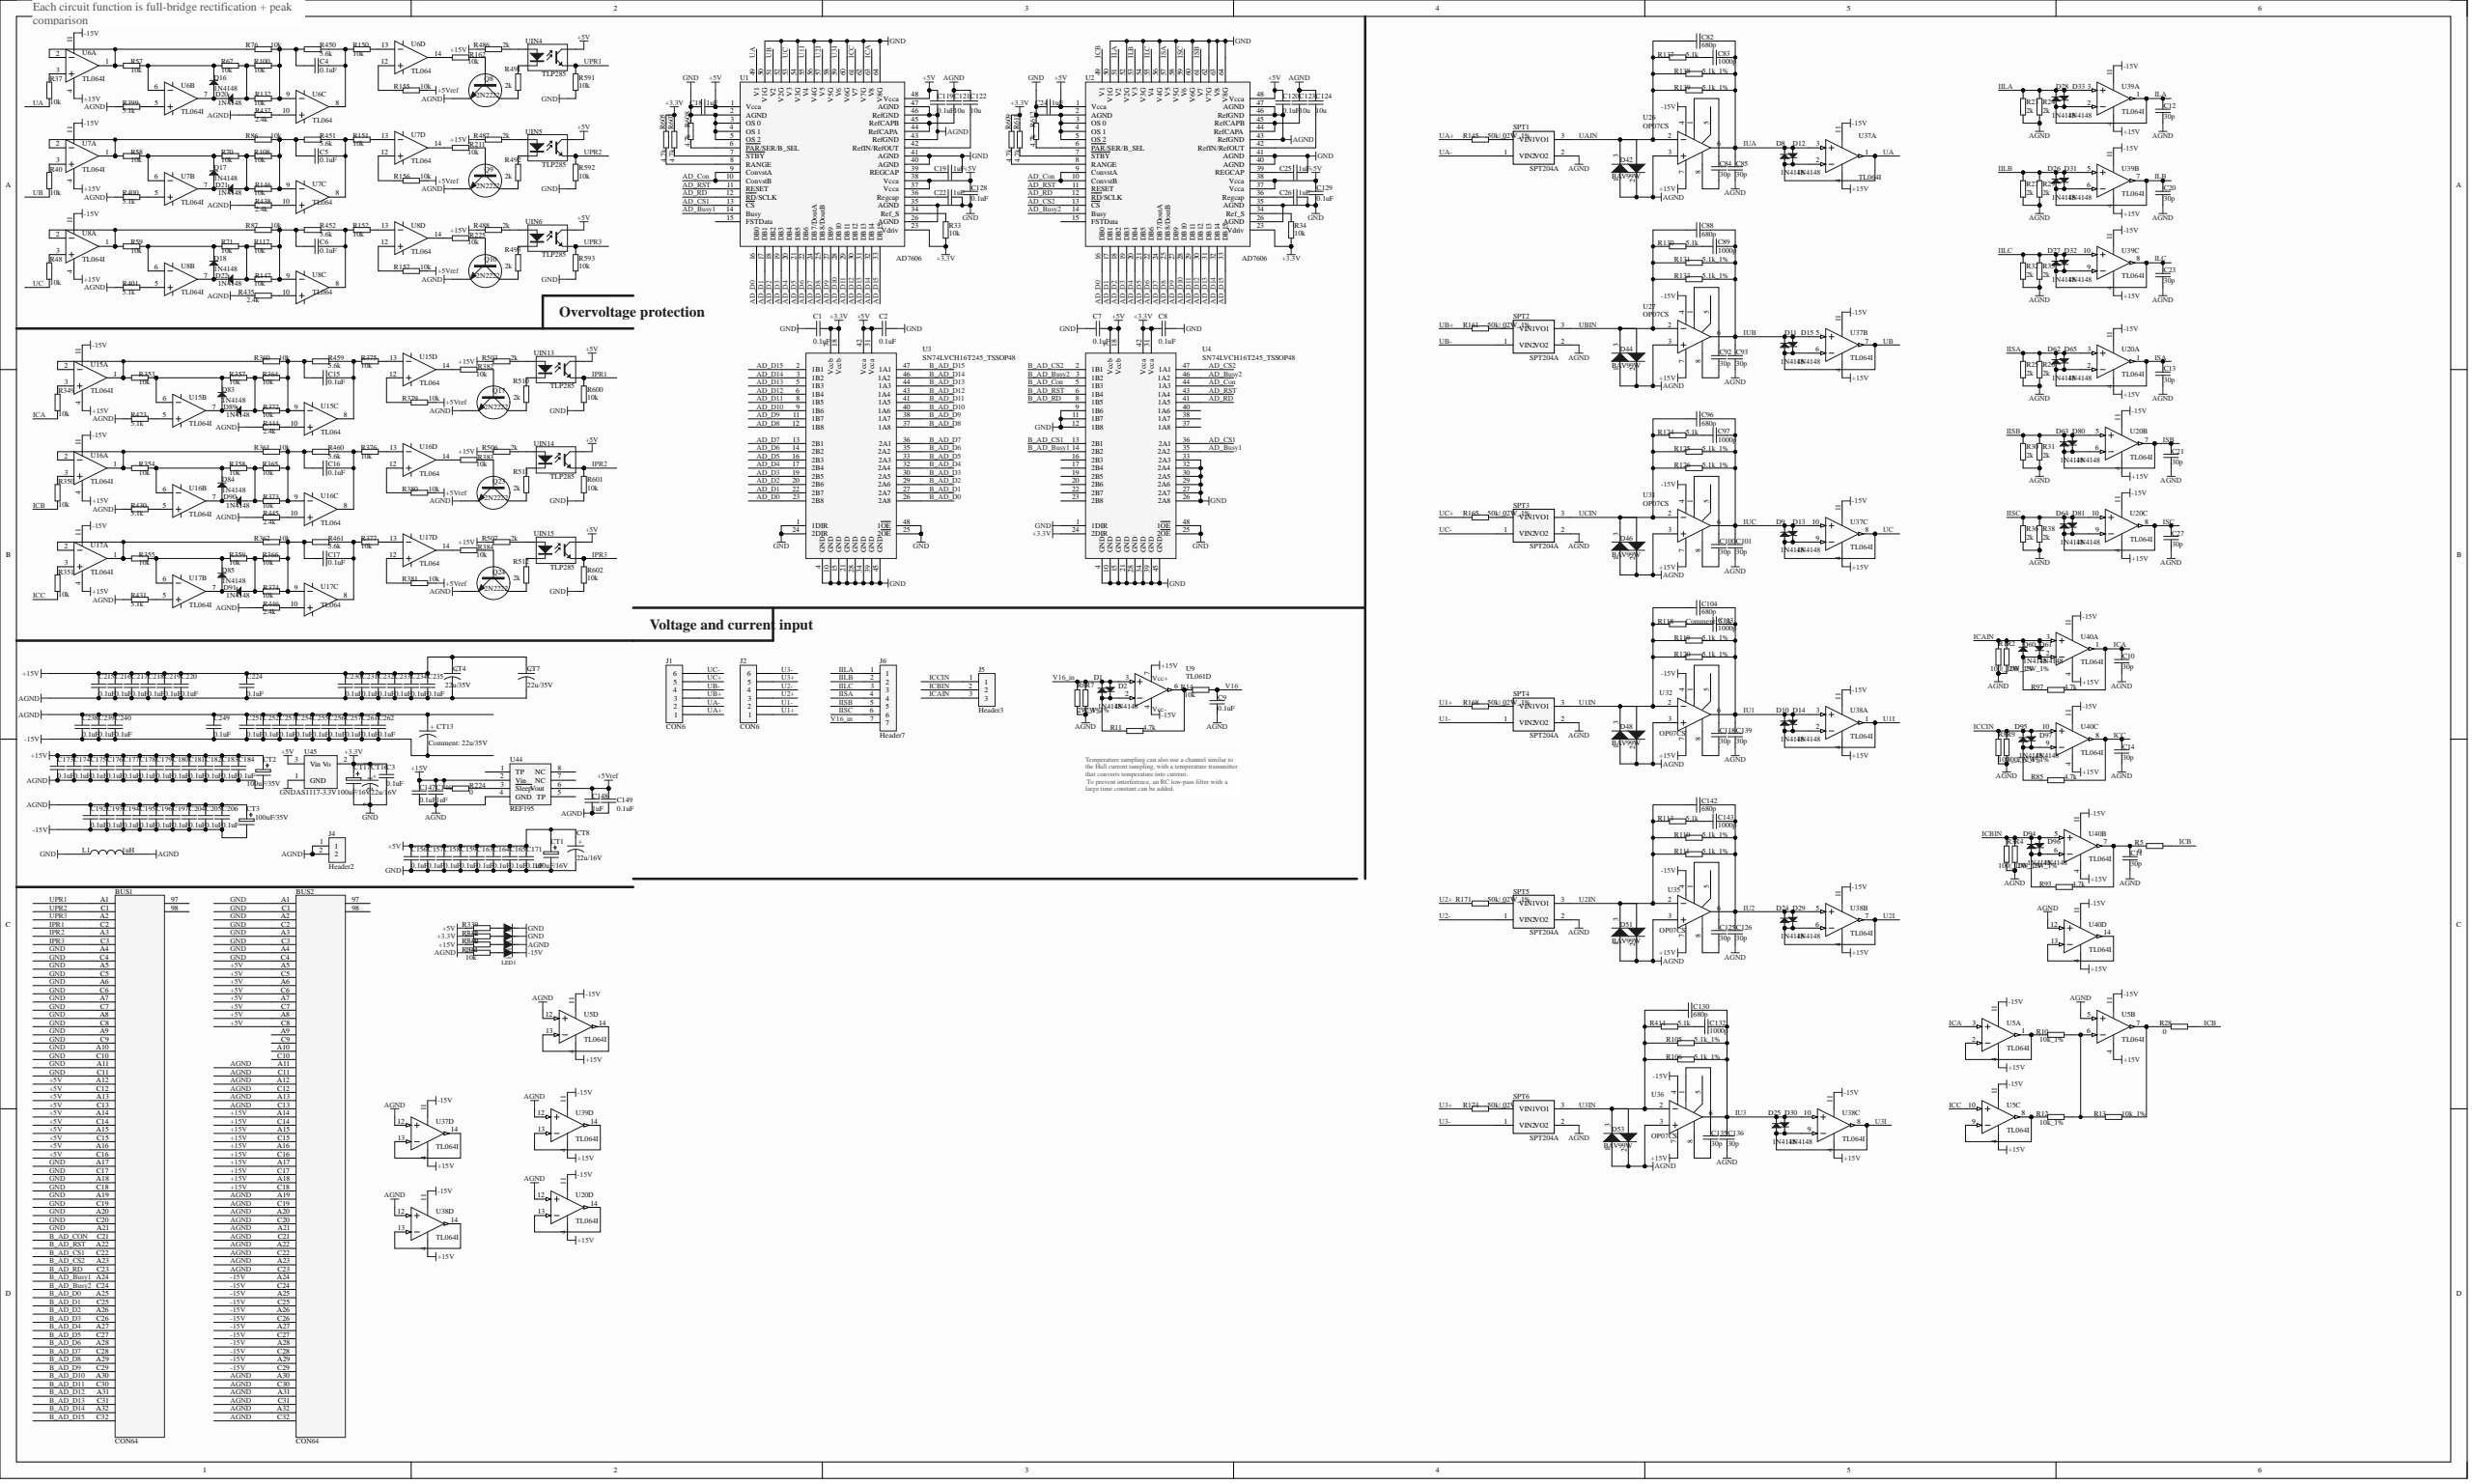Circuit board | Altium Designer | 386 parts | 266 nets
Bill of materials:
Comment,Description,Designator,Footprint,LibRef,Quantity
"CON64","Euro-style pin header, 64 positions","BUS1, BUS2","BUS64W-A","CON64","2"
"0.1uF","Capacitor, [NoValue]","C1, C2, C3, C4, C5, C6, C7, C8, C9, C15, C16, C17, C119, C120, C128, C129, C147, C149, C156, C157, C158, C159, C163, C164, C165, C171, C173, C174, C175, C176, C177, C178, C179, C180, C181, C182, C183, C184, C192, C193, C194, C195, C196, C197, C204, C205, C206, C215, C216, C217, C218, C219, C220, C224, C230, C231, C232, C233, C234, C235, C238, C239, C240, C249, C251, C252, C253, C254, C255, C256, C257, C261, C262","0603","CAP","73"
"30p","","C10, C11, C12, C13, C14, C20, C21, C23, C27, C84, C85, C92, C93, C100, C101, C118, C125, C126, C135, C136, C139","0603","CAP","21"
"1uF","Capacitor, [NoValue]","C18, C19, C22, C24, C25, C26, C146, C148","0603","CAP","8"
"680p","","C82, C88, C96, C104, C130, C142","0603","CAP","6"
"1000p","","C83, C89, C97, C113, C132, C143","0603","CAP","6"
"10u","Capacitor","C121, C122, C123, C124","0805","CAP","4"
"100uF/16V","","CT1, CT17","L470UF","EC","2"
"100uF/35V","","CT2, CT3","L470UF","EC","2"
"22u/35V","Capacitor","CT4, CT7, CT13","7343_CASE-D","CAPACITOR POL","3"
"22u/16V","Capacitor","CT8, CT16","3528_CASE-B","CAPACITOR POL","2"
"1N4148","","D1, D2, D8, D9, D10, D11, D12, D13, D14, D15, D16, D17, D18, D20, D21, D22, D24, D25, D26, D27, D28, D29, D30, D31, D32, D33, D60, D61, D62, D63, D64, D65, D80, D81, D83, D84, D85, D89, D90, D91, D94, D95, D96, D97","1N4148-A","DIODE-S","44"
"BAV99W","","D42, D44, D46, D48, D51, D53","SOT23R","DDIODEB","6"
"CON6","Connector","J1, J2","EDGCon_6P_5.08mm_ear","CON6","2"
"Header2","Header2","J4","EDGCON_2p_5.08mm_ear","Header2","1"
"Header3","Header3","J5","EDGCON_3p_5.08mm_ear","Header3","1"
"Header7","Header7","J6","EDGCon_7P_5.08mm_ear","Header7","1"
"1uH","","L1","0805","INDUCTOR","1"
"LEDGroup_4","LEDGroup_4","LED1","LEDGroup_4","LEDGroup_4","1"
"2N2222","NPN Transistor","Q8, Q9, Q10, Q17, Q23, Q24","SOT23-3","NPN","6"
"100|¸_2W_1%","","R1, R2, R3, R4, R8, R9","AXIAL0.8","RES2","6"
"0","","R5, R28, R224","0603","RES2","3"
"2W_1%","","R6, R7","AXIAL0.8","RES2","2"
"10k_1%","","R10, R12, R13","0603","RES2","3"
"4.7k","","R11, R85, R93, R97, R605, R607, R608, R609, R611, R612","0603","RES2","10"
"10k","","R14, R33, R34, R37, R40, R48, R57, R58, R59, R67, R70, R71, R76, R86, R87, R100, R108, R117, R132, R146, R147, R150, R151, R152, R155, R156, R157, R162, R211, R225, R340, R341, R349, R350, R351, R353, R354, R355, R357, R358, R359, R360, R361, R362, R364, R365, R366, R372, R373, R374, R375, R376, R377, R379, R380, R381, R382, R383, R384, R591, R592, R593, R600, R601, R602","0603","RES2","65"
"2k","","R23, R24, R25, R26, R27, R29, R30, R31, R32, R35, R36, R38","0805","RES2","12"
"5.1k_1%","","R105, R106, R110, R111, R119, R120, R125, R126, R131, R133, R138, R139","0603","RES2","12"
"5.1k","","R113, R118, R124, R130, R137, R399, R400, R401, R414, R423, R430, R431","0603","RES2","12"
"50k|¸_2W_1%","","R145, R161, R165, R168, R171, R174","AXIAL0.8","RES2","6"
"3.3k","","R339, R342","0603","RES2","2"
"2.4k","","R435, R437, R438, R444, R445, R446","0603","RES2","6"
"5.6k","","R450, R451, R452, R459, R460, R461","0603","RES2","6"
"2k","","R486, R487, R488, R491, R492, R493, R503, R506, R507, R510, R511, R512","0603","RES2","12"
"SPT204A","","SPT1, SPT2, SPT3, SPT4, SPT5, SPT6","SPT204A","SPT","6"
"AD7606","","U1, U2","AD7606_LQFP64","AD7606","2"
"SN74LVCH16T245_TSSOP48","TI SN74LVCH16T245DGGR","U3, U4","SN74LVC16245_TSSOP48","SN74LVCH16T245","2"
"TL064I","Low Power Quad Operational Amplifier, [NoValue]","U5, U6, U7, U8, U15, U16, U17, U20, U37, U38, U39, U40","TL064D_SOIC-14","TL064I, TL084","12"
"TL061D","TL061D","U9","TL061_SOIC8","TL061D","1"
"OP07CS","","U26, U27, U31, U32, U35, U36","SO-8","LM101","6"
"REF195","U?","U44","SO-8","REF195","1"
"AS1117-3.3V","","U45","SOT223","7810","1"
"TLP285","Optoisolator","UIN4, UIN5, UIN6, UIN13, UIN14, UIN15","TLP285_SOP4","521-1","6"
Netlist (Protel format):
[
BUS1
BUS64W-A
CON64



]
[
BUS2
BUS64W-A
CON64



]
[
C1
0603
0.1uF



]
[
C2
0603
0.1uF



]
[
C3
0603
0.1uF



]
[
C4
0603
0.1uF



]
[
C5
0603
0.1uF



]
[
C6
0603
0.1uF



]
[
C7
0603
0.1uF



]
[
C8
0603
0.1uF



]
[
C9
0603
0.1uF



]
[
C10
0603
30p



]
[
C11
0603
30p



]
[
C12
0603
30p



]
[
C13
0603
30p



]
[
C14
0603
30p



]
[
C15
0603
0.1uF



]
[
C16
0603
0.1uF



]
[
C17
0603
0.1uF



]
[
C18
0603
1uF



]
[
C19
0603
1uF



]
[
C20
0603
30p



]
[
C21
0603
30p



]
[
C22
0603
1uF



]
[
C23
0603
30p



]
[
C24
0603
1uF



]
[
C25
0603
1uF



]
[
C26
0603
1uF



]
[
C27
0603
30p



]
[
C82
0603
680p



]
[
C83
0603
1000p



]
[
C84
0603
30p



]
[
C85
0603
30p



]
[
C88
0603
680p



]
[
C89
0603
1000p



]
[
C92
0603
30p



]
[
C93
0603
30p



]
[
C96
0603
680p



]
[
C97
0603
1000p



]
[
C100
0603
30p



]
[
C101
0603
30p



]
[
C104
0603
680p



]
[
C113
0603
1000p



]
[
C118
0603
30p



]
[
C119
0603
0.1uF



]
[
C120
0603
0.1uF



]
[
C121
0805
10u



]
[
C122
0805
10u



]
[
C123
0805
10u



]
[
C124
0805
10u



]
[
C125
0603
30p



]
[
C126
0603
30p



]
[
C128
0603
0.1uF



]
[
C129
0603
0.1uF



]
[
C130
0603
680p



]
[
C132
0603
1000p



]
[
C135
0603
30p



]
[
C136
0603
30p



]
[
C139
0603
30p



]
[
C142
0603
680p



]
[
C143
0603
1000p



]
[
C146
0603
1uF



]
[
C147
0603
0.1uF



]
[
C148
0603
1uF



]
[
C149
0603
0.1uF



]
[
C156
0603
0.1uF



]
[
C157
0603
0.1uF



]
[
C158
0603
0.1uF



]
[
C159
0603
0.1uF



]
[
C163
0603
0.1uF



]
[
C164
0603
0.1uF



]
[
C165
0603
0.1uF



]
[
C171
0603
0.1uF



]
[
C173
0603
0.1uF



]
[
C174
0603
0.1uF



]
[
C175
0603
0.1uF



]
[
C176
0603
0.1uF



]
[
C177
0603
0.1uF



]
[
C178
0603
0.1uF



]
[
C179
0603
0.1uF



]
[
C180
0603
0.1uF



]
[
C181
0603
0.1uF



]
[
C182
0603
0.1uF



]
[
C183
0603
0.1uF



]
[
C184
0603
0.1uF



]
[
C192
0603
0.1uF



]
[
C193
0603
0.1uF



]
[
C194
0603
0.1uF



]
[
C195
0603
0.1uF



]
[
C196
0603
0.1uF



]
[
C197
0603
0.1uF



]
[
C204
0603
0.1uF



]
[
C205
0603
0.1uF



]
[
C206
0603
0.1uF



]
[
C215
0603
0.1uF



]
[
C216
0603
0.1uF



]
[
C217
0603
0.1uF



]
[
C218
0603
0.1uF



]
[
C219
0603
0.1uF



]
[
C220
0603
0.1uF



]
[
C224
0603
0.1uF



]
[
C230
0603
0.1uF



]
[
C231
0603
0.1uF



]
[
C232
0603
0.1uF



]
[
C233
0603
0.1uF



]
[
C234
0603
0.1uF



]
[
C235
0603
0.1uF



]
[
C238
0603
0.1uF



]
[
C239
0603
0.1uF



]
[
C240
0603
0.1uF



]
[
C249
0603
0.1uF



]
[
C251
0603
0.1uF



]
[
C252
0603
0.1uF



]
[
C253
0603
0.1uF



]
[
C254
0603
0.1uF



]
[
C255
0603
0.1uF



]
[
C256
0603
0.1uF



]
[
C257
0603
0.1uF



]
[
C261
0603
0.1uF



]
[
C262
0603
0.1uF



]
[
CT1
L470UF
100uF/16V



]
[
CT2
L470UF
100uF/35V



]
[
CT3
L470UF
100uF/35V



]
[
CT4
7343_CASE-D
22u/35V



]
[
CT7
7343_CASE-D
22u/35V



]
[
CT8
3528_CASE-B
22u/16V



]
[
CT13
7343_CASE-D
22u/35V



]
[
CT16
3528_CASE-B
22u/16V



]
[
CT17
L470UF
100uF/16V



]
[
D1
1N4148-A
1N4148



]
[
D2
1N4148-A
1N4148



]
[
D8
1N4148-A
1N4148



]
[
D9
1N4148-A
1N4148



]
[
D10
1N4148-A
1N4148



]
[
D11
1N4148-A
1N4148



]
[
D12
1N4148-A
1N4148



]
[
D13
1N4148-A
1N4148



]
[
D14
1N4148-A
1N4148



]
[
D15
1N4148-A
1N4148



]
[
D16
1N4148-A
1N4148



]
[
D17
1N4148-A
1N4148



]
[
D18
1N4148-A
1N4148



]
[
D20
1N4148-A
1N4148



]
[
D21
1N4148-A
1N4148



]
[
D22
1N4148-A
1N4148



]
[
D24
1N4148-A
1N4148



]
[
D25
1N4148-A
1N4148



]
[
D26
1N4148-A
1N4148



]
[
D27
1N4148-A
1N4148



]
[
D28
1N4148-A
1N4148



]
[
D29
1N4148-A
1N4148



]
[
D30
1N4148-A
1N4148



]
[
D31
1N4148-A
1N4148



]
[
D32
1N4148-A
1N4148



]
[
D33
1N4148-A
1N4148



]
[
D42
SOT23R
BAV99W



]
[
D44
SOT23R
BAV99W



]
[
D46
SOT23R
BAV99W



]
[
D48
SOT23R
BAV99W



]
[
D51
SOT23R
BAV99W



]
[
D53
SOT23R
BAV99W



]
[
D60
1N4148-A
1N4148



]
[
D61
1N4148-A
1N4148



]
[
D62
1N4148-A
1N4148



]
[
D63
1N4148-A
1N4148



]
[
D64
1N4148-A
1N4148



]
[
D65
1N4148-A
1N4148



]
[
D80
1N4148-A
1N4148



]
[
D81
1N4148-A
1N4148



]
[
D83
1N4148-A
1N4148



]
[
D84
1N4148-A
1N4148



]
[
D85
1N4148-A
1N4148



]
[
D89
1N4148-A
1N4148



]
[
D90
1N4148-A
1N4148



]
[
D91
1N4148-A
1N4148



]
[
D94
1N4148-A
1N4148



]
[
D95
1N4148-A
1N4148



]
[
D96
1N4148-A
1N4148



]
[
D97
1N4148-A
1N4148



]
[
J1
EDGCon_6P_5.08mm_ear
CON6



]
[
J2
EDGCon_6P_5.08mm_ear
CON6



]
[
J4
EDGCON_2p_5.08mm_ear
Header2



]
[
J5
EDGCON_3p_5.08mm_ear
Header3



]
[
J6
EDGCon_7P_5.08mm_ear
Header7



]
[
L1
0805
1uH



]
[
LED1
LEDGroup_4
LEDGroup_4



]
[
Q8
SOT23-3
2N2222



]
[
Q9
SOT23-3
2N2222



]
[
Q10
SOT23-3
2N2222



]
[
Q17
SOT23-3
2N2222



]
[
Q23
SOT23-3
2N2222



]
[
Q24
SOT23-3
2N2222



]
[
R1
AXIAL0.8
100|¸_2W_1%



]
[
R2
AXIAL0.8
100|¸_2W_1%



]
[
R3
AXIAL0.8
100|¸_2W_1%



]
[
R4
AXIAL0.8
100|¸_2W_1%



]
[
R5
0603
0



]
[
R6
AXIAL0.8
2W_1%



]
[
R7
AXIAL0.8
2W_1%



]
[
R8
AXIAL0.8
100|¸_2W_1%



]
[
R9
AXIAL0.8
100|¸_2W_1%



]
[
R10
0603
10k_1%



]
[
R11
0603
4.7k



]
[
R12
0603
10k_1%



]
[
R13
0603
10k_1%



]
[
R14
0603
10k



]
[
R23
0805
2k



]
[
R24
0805
2k



]
[
R25
0805
2k



]
[
R26
0805
2k



]
[
R27
0805
2k



]
[
R28
0603
0



]
[
R29
0805
2k



]
[
R30
0805
2k



]
[
R31
0805
2k



]
[
R32
0805
2k



]
[
R33
0603
10k



]
[
R34
0603
10k



]
[
R35
0805
2k



]
[
R36
0805
2k



]
[
R37
0603
10k



]
[
R38
0805
2k



]
[
R40
0603
10k



]
[
R48
0603
10k



]
[
R57
0603
10k



]
[
R58
0603
10k



]
[
R59
0603
10k



]
[
R67
0603
10k



]
[
R70
0603
10k



]
[
R71
0603
10k



]
[
R76
0603
10k



]
[
R85
0603
4.7k



]
[
R86
0603
10k



]
[
R87
0603
10k



]
[
R93
0603
4.7k



]
[
R97
0603
4.7k



]
[
R100
0603
10k



]
[
R105
0603
5.1k_1%



]
[
R106
0603
5.1k_1%



]
[
R108
0603
10k



]
[
R110
0603
5.1k_1%



]
[
R111
0603
5.1k_1%



]
[
R113
0603
5.1k



]
[
R117
0603
10k



]
[
R118
0603
5.1k



]
[
R119
0603
5.1k_1%



]
[
R120
0603
5.1k_1%



]
[
R124
0603
5.1k



]
[
R125
0603
5.1k_1%



]
[
R126
0603
5.1k_1%



]
[
R130
0603
5.1k



]
[
R131
0603
5.1k_1%



]
[
R132
0603
10k



]
[
R133
0603
5.1k_1%



]
[
R137
0603
5.1k



]
[
R138
0603
5.1k_1%



]
[
R139
0603
5.1k_1%



]
[
R145
AXIAL0.8
50k|¸_2W_1%



]
[
R146
0603
10k



]
[
R147
0603
10k



]
[
R150
0603
10k



]
[
R151
0603
10k



]
[
R152
0603
10k



]
[
R155
0603
10k



]
[
R156
0603
10k



]
[
R157
0603
10k



]
[
R161
AXIAL0.8
50k|¸_2W_1%



]
[
R162
0603
10k



]
[
R165
AXIAL0.8
50k|¸_2W_1%



]
[
R168
AXIAL0.8
50k|¸_2W_1%



]
[
R171
AXIAL0.8
50k|¸_2W_1%



]
[
R174
AXIAL0.8
50k|¸_2W_1%



]
[
R211
0603
10k



]
[
R224
0603
0



]
[
R225
0603
10k



]
[
R339
0603
3.3k



]
[
R340
0603
10k



]
[
R341
0603
10k



]
[
R342
0603
3.3k



]
[
R349
0603
10k



]
[
R350
0603
10k



]
[
R351
0603
10k



]
[
R353
0603
10k



]
[
R354
0603
10k



]
[
R355
0603
10k



]
[
R357
0603
10k



]
[
R358
0603
10k



]
[
R359
0603
10k



]
[
R360
0603
10k



]
[
R361
0603
10k



]
[
R362
0603
10k



]
[
R364
0603
10k



]
[
R365
0603
10k



]
[
R366
0603
10k



]
[
R372
0603
10k



]
[
R373
0603
10k



]
[
R374
0603
10k



]
[
R375
0603
10k



]
[
R376
0603
10k



]
[
R377
0603
10k



]
[
R379
0603
10k



]
[
R380
0603
10k



]
[
R381
0603
10k



]
[
R382
0603
10k



]
[
R383
0603
10k



]
[
R384
0603
10k



]
[
R399
0603
5.1k



]
[
R400
0603
5.1k



]
[
R401
0603
5.1k



]
[
R414
0603
5.1k



]
[
R423
0603
5.1k



]
[
R430
0603
5.1k



]
[
R431
0603
5.1k



]
[
R435
0603
2.4k



]
[
R437
0603
2.4k



]
[
R438
0603
2.4k



]
[
R444
0603
2.4k



]
[
R445
0603
2.4k



]
[
R446
0603
2.4k



]
[
R450
0603
5.6k



]
[
R451
0603
5.6k



]
[
R452
0603
5.6k



]
[
R459
0603
5.6k



]
[
R460
0603
5.6k



]
[
R461
0603
5.6k



]
[
R486
0603
2k



]
[
R487
0603
2k



]
[
R488
0603
2k



]
[
R491
0603
2k



]
[
R492
0603
2k



]
[
R493
0603
2k



]
[
R503
0603
2k



]
[
R506
0603
2k



]
[
R507
0603
2k



]
[
R510
0603
2k



]
[
R511
0603
2k



]
[
R512
0603
2k



]
[
R591
0603
10k



]
[
R592
0603
10k



]
[
R593
0603
10k



]
[
R600
0603
10k



]
[
R601
0603
10k



]
[
R602
0603
10k



]
[
R605
0603
4.7k



]
[
R607
0603
4.7k



]
[
R608
0603
4.7k



]
[
R609
0603
4.7k



]
[
R611
0603
4.7k



]
[
R612
0603
4.7k



]
[
SPT1
SPT204A
SPT204A



]
[
SPT2
SPT204A
SPT204A



]
[
SPT3
SPT204A
SPT204A



]
[
SPT4
SPT204A
SPT204A



]
[
SPT5
SPT204A
SPT204A



]
[
SPT6
SPT204A
SPT204A



]
[
U1
AD7606_LQFP64
AD7606



]
[
U2
AD7606_LQFP64
AD7606



]
[
U3
SN74LVC16245_TSSOP48
SN74LVCH16T245_TSSOP48



]
[
U4
SN74LVC16245_TSSOP48
SN74LVCH16T245_TSSOP48



]
[
U5
TL064D_SOIC-14
TL064I



]
[
U6
TL064D_SOIC-14
TL064I



]
[
U7
TL064D_SOIC-14
TL064I



]
[
U8
TL064D_SOIC-14
TL064I



]
[
U9
TL061_SOIC8
TL061D



]
[
U15
TL064D_SOIC-14
TL064I



]
[
U16
TL064D_SOIC-14
TL064I



]
[
U17
TL064D_SOIC-14
TL064I



]
[
U20
TL064D_SOIC-14
TL064I



]
[
U26
SO-8
OP07CS



]
[
U27
SO-8
OP07CS



]
[
U31
SO-8
OP07CS



]
[
U32
SO-8
OP07CS



]
[
U35
SO-8
OP07CS



]
[
U36
SO-8
OP07CS



]
[
U37
TL064D_SOIC-14
TL064I



]
[
U38
TL064D_SOIC-14
TL064I



]
[
U39
TL064D_SOIC-14
TL064I



]
[
U40
TL064D_SOIC-14
TL064I



]
[
U44
SO-8
REF195



]
[
U45
SOT223
AS1117-3.3V



]
[
UIN4
TLP285_SOP4
TLP285



]
[
UIN5
TLP285_SOP4
TLP285



]
[
UIN6
TLP285_SOP4
TLP285



]
[
UIN13
TLP285_SOP4
TLP285



]
[
UIN14
TLP285_SOP4
TLP285



]
[
UIN15
TLP285_SOP4
TLP285



]
(
V16_in
D1-K
D2-A
J6-7
R6-2
R7-2
U9-3
)
(
V16
C9-2
R14-1
)
(
UPR3
BUS1-A2
R593-2
UIN6-3
)
(
UPR2
BUS1-C1
R592-2
UIN5-3
)
(
UPR1
BUS1-A1
R591-2
UIN4-3
)
(
UCIN
C96-2
D46-3
R124-2
R125-2
R126-2
SPT3-3
U31-2
)
(
UC-
J1-6
SPT3-1
)
(
UC+
J1-5
R165-2
)
(
UC
D9-A
D13-K
R48-2
U1-53
U37-8
U37-9
)
(
UBIN
C88-2
D44-3
R130-2
R131-2
R133-2
SPT2-3
U27-2
)
(
UB-
J1-4
SPT2-1
)
(
UB+
J1-3
R161-2
)
(
UB
D11-A
D15-K
R40-2
U1-51
U37-6
U37-7
)
(
UAIN
C82-2
D42-3
R137-2
R138-2
R139-2
SPT1-3
U26-2
)
(
UA-
J1-2
SPT1-1
)
(
UA+
J1-1
R145-2
)
(
UA
D8-A
D12-K
R37-2
U1-49
U37-1
U37-2
)
(
U3IN
C130-2
D53-3
R105-2
R106-2
R414-2
SPT6-3
U36-2
)
(
U3I
D25-A
D30-K
U1-59
U38-8
U38-9
)
(
U3-
J2-6
SPT6-1
)
(
U3+
J2-5
R174-2
)
(
U2IN
C142-2
D51-3
R110-2
R111-2
R113-2
SPT5-3
U35-2
)
(
U2I
D24-A
D29-K
U1-57
U38-6
U38-7
)
(
U2-
J2-4
SPT5-1
)
(
U2+
J2-3
R171-2
)
(
U1IN
C104-2
D48-3
R118-2
R119-2
R120-2
SPT4-3
U32-2
)
(
U1I
D10-A
D14-K
U1-55
U38-1
U38-2
)
(
U1-
J2-2
SPT4-1
)
(
U1+
J2-1
R168-2
)
(
NetU40_13
U40-13
U40-14
)
(
NetU39_13
U39-13
U39-14
)
(
NetU38_13
U38-13
U38-14
)
(
NetU37_13
U37-13
U37-14
)
(
NetU20_13
U20-13
U20-14
)
(
NetU5_13
U5-13
U5-14
)
(
NetR612_1
R612-1
U2-6
)
(
NetR611_1
R611-1
U2-7
)
(
NetR609_1
R609-1
U2-8
)
(
NetR608_1
R608-1
U1-6
)
(
NetR607_1
R607-1
U1-7
)
(
NetR605_1
R605-1
U1-8
)
(
NetR512_1
R512-1
UIN15-2
)
(
NetR511_1
R511-1
UIN14-2
)
(
NetR510_1
R510-1
UIN13-2
)
(
NetR507_2
R507-2
UIN15-1
)
(
NetR506_2
R506-2
UIN14-1
)
(
NetR503_2
R503-2
UIN13-1
)
(
NetR493_1
R493-1
UIN6-2
)
(
NetR492_1
R492-1
UIN5-2
)
(
NetR491_1
R491-1
UIN4-2
)
(
NetR488_2
R488-2
UIN6-1
)
(
NetR487_2
R487-2
UIN5-1
)
(
NetR486_2
R486-2
UIN4-1
)
(
NetR446_1
R446-1
U17-10
)
(
NetR445_1
R445-1
U16-10
)
(
NetR444_1
R444-1
U15-10
)
(
NetR438_1
R438-1
U7-10
)
(
NetR437_1
R437-1
U6-10
)
(
NetR435_1
R435-1
U8-10
)
(
NetR431_1
R431-1
U17-5
)
(
NetR430_1
R430-1
U16-5
)
(
NetR423_1
R423-1
U15-5
)
(
NetR401_1
R401-1
U8-5
)
(
NetR400_1
R400-1
U7-5
)
(
NetR399_1
R399-1
U6-5
)
(
NetR384_2
R384-2
U17-14
)
(
NetR383_2
R383-2
U16-14
)
(
NetR382_2
R382-2
U15-14
)
(
NetR381_1
R381-1
U17-12
)
(
NetR380_1
R380-1
U16-12
)
(
NetR379_1
R379-1
U15-12
)
(
NetR377_1
R377-1
U17-13
)
(
NetR376_1
R376-1
U16-13
)
(
NetR375_1
R375-1
U15-13
)
(
NetR355_2
R355-2
R362-2
U17-1
U17-2
)
(
NetR354_2
R354-2
R361-2
U16-1
U16-2
)
(
NetR353_2
R353-2
R360-2
U15-1
U15-2
)
(
NetR351_1
R351-1
U17-3
)
(
NetR350_1
R350-1
U16-3
)
(
NetR349_1
R349-1
U15-3
)
(
NetR225_2
R225-2
U8-14
)
(
NetR224_1
R224-1
U44-3
)
(
NetR211_2
R211-2
U7-14
)
(
NetR174_1
R174-1
SPT6-0
)
(
NetR171_1
R171-1
SPT5-0
)
(
NetR168_1
R168-1
SPT4-0
)
(
NetR165_1
R165-1
SPT3-0
)
(
NetR162_2
R162-2
U6-14
)
(
NetR161_1
R161-1
SPT2-0
)
(
NetR157_1
R157-1
U8-12
)
(
NetR156_1
R156-1
U7-12
)
(
NetR155_1
R155-1
U6-12
)
(
NetR152_1
R152-1
U8-13
)
(
NetR151_1
R151-1
U7-13
)
(
NetR150_1
R150-1
U6-13
)
(
NetR145_1
R145-1
SPT1-0
)
(
NetR59_2
R59-2
R87-2
U8-1
U8-2
)
(
NetR58_2
R58-2
R86-2
U7-1
U7-2
)
(
NetR57_2
R57-2
R76-2
U6-1
U6-2
)
(
NetR48_1
R48-1
U8-3
)
(
NetR40_1
R40-1
U7-3
)
(
NetR37_1
R37-1
U6-3
)
(
NetR34_1
R34-1
U2-34
)
(
NetR33_1
R33-1
U1-34
)
(
NetR13_1
R13-1
R28-2
U5-7
)
(
NetR12_2
R12-2
U5-8
U5-9
)
(
NetR11_1
R11-1
R14-2
U9-6
)
(
NetR10_2
R10-2
U5-1
U5-2
)
(
NetR10_1
R10-1
R12-1
R13-2
U5-6
)
(
NetQ24_C
Q24-C
R512-2
)
(
NetQ24_B
Q24-B
R384-1
)
(
NetQ23_C
Q23-C
R511-2
)
(
NetQ23_B
Q23-B
R383-1
)
(
NetQ17_C
Q17-C
R510-2
)
(
NetQ17_B
Q17-B
R382-1
)
(
NetQ10_C
Q10-C
R493-2
)
(
NetQ10_B
Q10-B
R225-1
)
(
NetQ9_C
Q9-C
R492-2
)
(
NetQ9_B
Q9-B
R211-1
)
(
NetQ8_C
Q8-C
R491-2
)
(
NetQ8_B
Q8-B
R162-1
)
(
NetLED1_7
LED1-7
R341-1
)
(
NetLED1_5
LED1-5
R340-1
)
(
NetLED1_3
LED1-3
R342-1
)
(
NetLED1_1
LED1-1
R339-1
)
(
NetD95_A
D95-A
D97-K
R85-2
U40-9
)
(
NetD94_A
D94-A
D96-K
R93-2
U40-6
)
(
NetD91_A
D91-A
R359-1
R366-2
R374-2
)
(
NetD90_A
D90-A
R358-1
R365-2
R373-2
)
(
NetD89_A
D89-A
R357-1
R364-2
R372-2
)
(
NetD85_K
D85-K
R355-1
R359-2
U17-6
)
(
NetD85_A
D85-A
D91-K
U17-7
)
(
NetD84_K
D84-K
R354-1
R358-2
U16-6
)
(
NetD84_A
D84-A
D90-K
U16-7
)
(
NetD83_K
D83-K
R353-1
R357-2
U15-6
)
(
NetD83_A
D83-A
D89-K
U15-7
)
(
NetD60_A
D60-A
D61-K
R97-2
U40-2
)
(
NetD22_A
D22-A
R71-1
R117-2
R147-2
)
(
NetD21_A
D21-A
R70-1
R108-2
R146-2
)
(
NetD20_A
D20-A
R67-1
R100-2
R132-2
)
(
NetD18_K
D18-K
R59-1
R71-2
U8-6
)
(
NetD18_A
D18-A
D22-K
U8-7
)
(
NetD17_K
D17-K
R58-1
R70-2
U7-6
)
(
NetD17_A
D17-A
D21-K
U7-7
)
(
NetD16_K
D16-K
R57-1
R67-2
U6-6
)
(
NetD16_A
D16-A
D20-K
U6-7
)
(
NetD1_A
D1-A
D2-K
R11-2
U9-2
)
(
NetC143_2
C143-2
R113-1
)
(
NetC135_2
C135-2
U36-1
)
(
NetC135_1
C135-1
U36-8
)
(
NetC132_2
C132-2
R414-1
)
(
NetC125_2
C125-2
U35-1
)
(
NetC125_1
C125-1
U35-8
)
(
NetC124_2
C124-2
U2-42
)
(
NetC123_2
C123-2
U2-44
U2-45
)
(
NetC122_2
C122-2
U1-42
)
(
NetC121_2
C121-2
U1-44
U1-45
)
(
NetC118_2
C118-2
U32-1
)
(
NetC118_1
C118-1
U32-8
)
(
NetC113_2
C113-2
R118-1
)
(
NetC100_2
C100-2
U31-1
)
(
NetC100_1
C100-1
U31-8
)
(
NetC97_2
C97-2
R124-1
)
(
NetC92_2
C92-2
U27-1
)
(
NetC92_1
C92-1
U27-8
)
(
NetC89_2
C89-2
R130-1
)
(
NetC84_2
C84-2
U26-1
)
(
NetC84_1
C84-1
U26-8
)
(
NetC83_2
C83-2
R137-1
)
(
NetC26_2
C26-2
U2-36
)
(
NetC25_2
C25-2
U2-39
)
(
NetC22_2
C22-2
U1-36
)
(
NetC19_2
C19-2
U1-39
)
(
NetC17_2
C17-2
R362-1
R366-1
R374-1
R461-2
U17-9
)
(
NetC17_1
C17-1
R377-2
R461-1
U17-8
)
(
NetC16_2
C16-2
R361-1
R365-1
R373-1
R460-2
U16-9
)
(
NetC16_1
C16-1
R376-2
R460-1
U16-8
)
(
NetC15_2
C15-2
R360-1
R364-1
R372-1
R459-2
U15-9
)
(
NetC15_1
C15-1
R375-2
R459-1
U15-8
)
(
NetC11_2
C11-2
R5-2
R93-1
U40-7
)
(
NetC6_2
C6-2
R87-1
R117-1
R147-1
R452-2
U8-9
)
(
NetC6_1
C6-1
R152-2
R452-1
U8-8
)
(
NetC5_2
C5-2
R86-1
R108-1
R146-1
R451-2
U7-9
)
(
NetC5_1
C5-1
R151-2
R451-1
U7-8
)
(
NetC4_2
C4-2
R76-1
R100-1
R132-1
R450-2
U6-9
)
(
NetC4_1
C4-1
R150-2
R450-1
U6-8
)
(
IUC
C96-1
C97-1
C101-2
D9-K
D13-A
R125-1
R126-1
U31-6
U37-10
)
(
IUB
C88-1
C89-1
C93-2
D11-K
D15-A
R131-1
R133-1
U27-6
U37-5
)
(
IUA
C82-1
C83-1
C85-2
D8-K
D12-A
R138-1
R139-1
U26-6
U37-3
)
(
IU3
C130-1
C132-1
C136-2
D25-K
D30-A
R105-1
R106-1
U36-6
U38-10
)
(
IU2
C126-2
C142-1
C143-1
D24-K
D29-A
R110-1
R111-1
U35-6
U38-5
)
(
IU1
C104-1
C113-1
C139-2
D10-K
D14-A
R119-1
R120-1
U32-6
U38-3
)
(
ISC
C27-2
D64-A
D81-K
U2-59
U20-8
U20-9
)
(
ISB
C21-2
D63-A
D80-K
U2-61
U20-6
U20-7
)
(
ISA
C13-2
D62-A
D65-K
U2-57
U20-1
U20-2
)
(
IPR3
BUS1-C3
R602-2
UIN15-3
)
(
IPR2
BUS1-A3
R601-2
UIN14-3
)
(
IPR1
BUS1-C2
R600-2
UIN13-3
)
(
ILC
C23-2
D27-A
D32-K
U2-55
U39-8
U39-9
)
(
ILB
C20-2
D26-A
D31-K
U2-53
U39-6
U39-7
)
(
ILA
C12-2
D28-A
D33-K
U2-51
U39-1
U39-2
)
(
IISC
D64-K
D81-A
J6-6
R36-1
R38-1
U20-10
)
(
IISB
D63-K
D80-A
J6-5
R30-1
R31-1
U20-5
)
(
IISA
D62-K
D65-A
J6-4
R25-1
R26-1
U20-3
)
(
IILC
D27-K
D32-A
J6-3
R32-1
R35-1
U39-10
)
(
IILB
D26-K
D31-A
J6-2
R27-1
R29-1
U39-5
)
(
IILA
D28-K
D33-A
J6-1
R23-1
R24-1
U39-3
)
(
ICCIN
D95-K
D97-A
J5-1
R8-2
R9-2
U40-10
)
(
ICC
C14-2
R85-1
R351-2
U1-61
U5-10
U40-8
)
(
ICBIN
D94-K
D96-A
J5-2
R3-2
R4-2
U40-5
)
(
ICB
R5-1
R28-1
R350-2
U2-49
)
(
ICAIN
D60-K
D61-A
J5-3
R1-2
R2-2
U40-3
)
(
ICA
C10-2
R97-1
R349-2
U1-63
U5-3
U40-1
)
(
GND
BUS1-A4
BUS1-A5
BUS1-A6
BUS1-A7
BUS1-A8
BUS1-A9
BUS1-A10
BUS1-A11
BUS1-A17
BUS1-A18
BUS1-A19
BUS1-A20
BUS1-A21
BUS1-C4
BUS1-C5
BUS1-C6
BUS1-C7
BUS1-C8
BUS1-C9
BUS1-C10
BUS1-C11
BUS1-C17
BUS1-C18
BUS1-C19
BUS1-C20
BUS2-A1
BUS2-A2
BUS2-A3
BUS2-A4
BUS2-C1
BUS2-C2
BUS2-C3
BUS2-C4
C1-1
C2-2
C3-2
C7-1
C8-2
C18-2
C19-1
C22-1
C24-2
C25-1
C26-1
C128-2
C129-2
C156-1
C157-2
C158-2
C159-1
C163-2
C164-2
C165-1
C171-2
CT1-2
CT8-2
CT16-2
CT17-2
L1-1
LED1-2
LED1-4
R591-1
R592-1
R593-1
R600-1
R601-1
R602-1
R608-2
R612-2
U1-2
U1-3
U1-4
U1-5
U1-26
U1-35
U1-40
U1-41
U1-50
U1-52
U1-54
U1-56
U1-58
U1-60
U1-62
U1-64
U2-2
U2-3
U2-4
U2-5
U2-26
U2-35
U2-40
U2-41
U2-50
U2-52
U2-54
U2-56
U2-58
U2-60
U2-62
U2-63
U2-64
U3-1
U3-4
U3-10
U3-15
U3-21
U3-24
U3-25
U3-28
U3-34
U3-39
U3-45
U3-48
U4-1
U4-4
U4-9
U4-10
U4-11
U4-12
U4-15
U4-21
U4-25
U4-26
U4-27
U4-28
U4-29
U4-30
U4-32
U4-33
U4-34
U4-39
U4-45
U4-48
U45-1
)
(
B_AD_RST
BUS1-A22
U4-6
)
(
B_AD_RD
BUS1-C23
U4-8
)
(
B_AD_D15
BUS1-C32
U3-47
)
(
B_AD_D14
BUS1-A32
U3-46
)
(
B_AD_D13
BUS1-C31
U3-44
)
(
B_AD_D12
BUS1-A31
U3-43
)
(
B_AD_D11
BUS1-C30
U3-41
)
(
B_AD_D10
BUS1-A30
U3-40
)
(
B_AD_D9
BUS1-C29
U3-38
)
(
B_AD_D8
BUS1-A29
U3-37
)
(
B_AD_D7
BUS1-C28
U3-36
)
(
B_AD_D6
BUS1-A28
U3-35
)
(
B_AD_D5
BUS1-C27
U3-33
)
(
B_AD_D4
BUS1-A27
U3-32
)
(
B_AD_D3
BUS1-C26
U3-30
)
(
B_AD_D2
BUS1-A26
U3-29
)
(
B_AD_D1
BUS1-C25
U3-27
)
(
B_AD_D0
BUS1-A25
U3-26
)
(
B_AD_CS2
BUS1-A23
U4-2
)
(
B_AD_CS1
BUS1-C22
U4-13
)
(
B_AD_Con
BUS1-C21
U4-5
)
(
B_AD_Busy2
BUS1-C24
U4-3
)
(
B_AD_Busy1
BUS1-A24
U4-14
)
(
AGND
BUS2-A11
BUS2-A12
BUS2-A13
BUS2-A19
BUS2-A20
BUS2-A21
BUS2-A22
BUS2-A23
BUS2-A30
BUS2-A31
BUS2-A32
BUS2-C11
BUS2-C12
BUS2-C13
BUS2-C19
BUS2-C20
BUS2-C21
BUS2-C22
BUS2-C23
BUS2-C30
BUS2-C31
BUS2-C32
C9-1
C10-1
C11-1
C12-1
C13-1
C14-1
C20-1
C21-1
C23-1
C27-1
C85-1
C93-1
C101-1
C119-2
C120-2
C121-1
C122-1
C123-1
C124-1
C126-1
C136-1
C139-1
C146-2
C147-2
C148-2
C149-1
C173-1
C174-2
C175-2
C176-1
C177-2
C178-1
C179-1
C180-2
C181-2
C182-1
C183-1
C184-2
C192-1
C193-2
C194-1
C195-2
C196-2
C197-1
C204-1
C205-1
C206-2
C215-2
C216-1
C217-1
C218-2
C219-1
C220-1
C224-2
C230-1
C231-2
C232-2
C233-1
C234-2
C235-1
C238-1
C239-2
C240-2
C249-2
C251-1
C252-2
C253-1
C254-2
C255-2
C256-1
C257-1
C261-1
C262-2
CT2-2
CT3-1
CT4-2
CT7-2
CT13-1
D42-1
D42-2
D44-1
D44-2
D46-1
D46-2
D48-1
D48-2
D51-1
D51-2
D53-1
D53-2
J4-1
J4-2
L1-2
LED1-6
Q8-E
Q9-E
Q10-E
Q17-E
Q23-E
Q24-E
R1-1
R2-1
R3-1
R4-1
R6-1
R7-1
R8-1
R9-1
R23-2
R24-2
R25-2
R26-2
R27-2
R29-2
R30-2
R31-2
R32-2
R35-2
R36-2
R38-2
R341-2
R399-2
R400-2
R401-2
R423-2
R430-2
R431-2
R435-2
R437-2
R438-2
R444-2
R445-2
R446-2
SPT1-2
SPT2-2
SPT3-2
SPT4-2
SPT5-2
SPT6-2
U1-43
U1-46
U1-47
U2-43
U2-46
U2-47
U5-5
U5-12
U20-12
U26-3
U27-3
U31-3
U32-3
U35-3
U36-3
U37-12
U38-12
U39-12
U40-12
U44-4
)
(
AD_RST
U1-11
U2-11
U4-43
)
(
AD_RD
U1-12
U2-12
U4-41
)
(
AD_D15
U1-33
U2-33
U3-2
)
(
AD_D14
U1-32
U2-32
U3-3
)
(
AD_D13
U1-31
U2-31
U3-5
)
(
AD_D12
U1-30
U2-30
U3-6
)
(
AD_D11
U1-29
U2-29
U3-8
)
(
AD_D10
U1-28
U2-28
U3-9
)
(
AD_D9
U1-27
U2-27
U3-11
)
(
AD_D8
U1-25
U2-25
U3-12
)
(
AD_D7
U1-24
U2-24
U3-13
)
(
AD_D6
U1-22
U2-22
U3-14
)
(
AD_D5
U1-21
U2-21
U3-16
)
(
AD_D4
U1-20
U2-20
U3-17
)
(
AD_D3
U1-19
U2-19
U3-19
)
(
AD_D2
U1-18
U2-18
U3-20
)
(
AD_D1
U1-17
U2-17
U3-22
)
(
AD_D0
U1-16
U2-16
U3-23
)
(
AD_CS2
U2-13
U4-47
)
(
AD_CS1
U1-13
U4-36
)
(
AD_Con
U1-9
U1-10
U2-9
U2-10
U4-44
)
(
AD_Busy2
U2-14
U4-46
)
(
AD_Busy1
U1-14
U4-35
)
(
-15V
BUS2-A24
BUS2-A25
BUS2-A26
BUS2-A27
BUS2-A28
BUS2-A29
BUS2-C24
BUS2-C25
BUS2-C26
BUS2-C27
BUS2-C28
BUS2-C29
C192-2
C193-1
C194-2
C195-1
C196-1
C197-2
C204-2
C205-2
C206-1
C238-2
C239-1
C240-1
C249-1
C251-2
C252-1
C253-2
C254-1
C255-1
C256-2
C257-2
C261-2
C262-1
CT3-2
CT13-2
LED1-8
U5-11
U6-11
U7-11
U8-11
U9-4
U15-11
U16-11
U17-11
U20-11
U26-4
U27-4
U31-4
U32-4
U35-4
U36-4
U37-11
U38-11
U39-11
U40-11
)
(
+15V
BUS2-A14
BUS2-A15
BUS2-A16
BUS2-A17
BUS2-A18
BUS2-C14
BUS2-C15
BUS2-C16
BUS2-C17
BUS2-C18
C146-1
C147-1
C173-2
C174-1
C175-1
C176-2
C177-1
C178-2
C179-2
C180-1
C181-1
C182-2
C183-2
C184-1
C215-1
C216-2
C217-2
C218-1
C219-2
C220-2
C224-1
C230-2
C231-1
C232-1
C233-2
C234-1
C235-2
CT2-1
CT4-1
CT7-1
R224-2
R340-2
R486-1
R487-1
R488-1
R503-1
R506-1
R507-1
U5-4
U6-4
U7-4
U8-4
U9-7
U15-4
U16-4
U17-4
U20-4
U26-7
U27-7
U31-7
U32-7
U35-7
U36-7
U37-4
U38-4
U39-4
U40-4
U44-2
)
(
+5Vref
C148-1
C149-2
R155-2
R156-2
R157-2
R379-2
R380-2
R381-2
U44-6
)
(
+5V
BUS1-A12
BUS1-A13
BUS1-A14
BUS1-A15
BUS1-A16
BUS1-C12
BUS1-C13
BUS1-C14
BUS1-C15
BUS1-C16
BUS2-A5
BUS2-A6
BUS2-A7
BUS2-A8
BUS2-C5
BUS2-C6
BUS2-C7
BUS2-C8
C2-1
C7-2
C18-1
C24-1
C119-1
C120-1
C128-1
C129-1
C156-2
C157-1
C158-1
C159-2
C163-1
C164-1
C165-2
C171-1
CT1-1
CT8-1
R339-2
U1-1
U1-37
U1-38
U1-48
U2-1
U2-37
U2-38
U2-48
U3-31
U3-42
U4-7
U4-18
U45-3
UIN4-4
UIN5-4
UIN6-4
UIN13-4
UIN14-4
UIN15-4
)
(
+3.3V
C1-2
C3-1
C8-1
CT16-1
CT17-1
R33-2
R34-2
R342-2
R605-2
R607-2
R609-2
R611-2
U1-23
U2-23
U3-7
U3-18
U4-24
U4-31
U4-42
U45-2
)